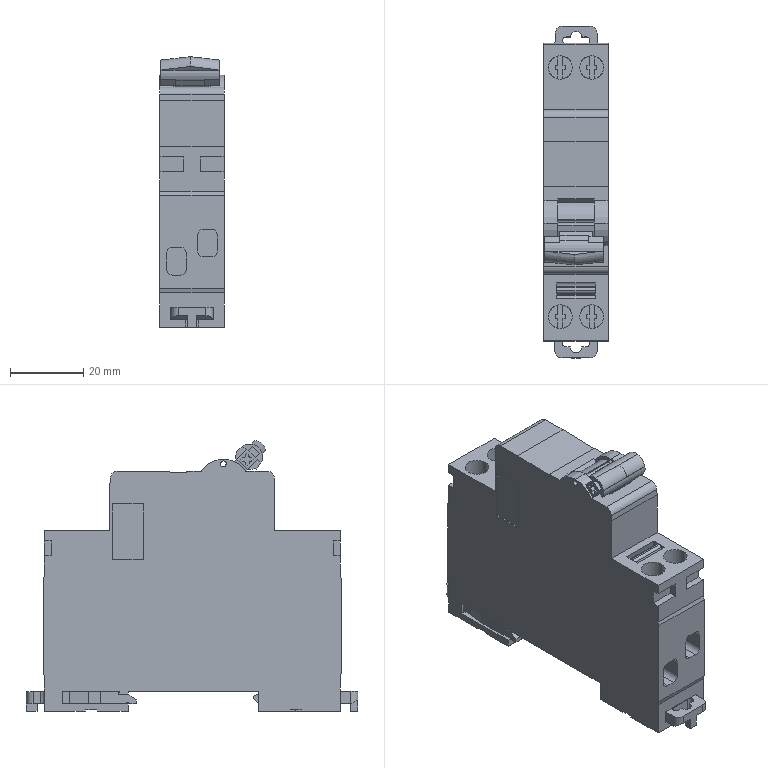Part | STEP file | Schneider miniature circuit breaker iDPNN-1P+N-C10A | 1 solid | 480 faces | box 17.5 x 90.6 x 73.848 mm | volume 76092 mm3 | plane 377 | cylinder 101 | spline 2 | commonest cylinder face diameters 4 x15 1.278 x12 1.6 x11 2 x10 3.2 x9 6.5 x8